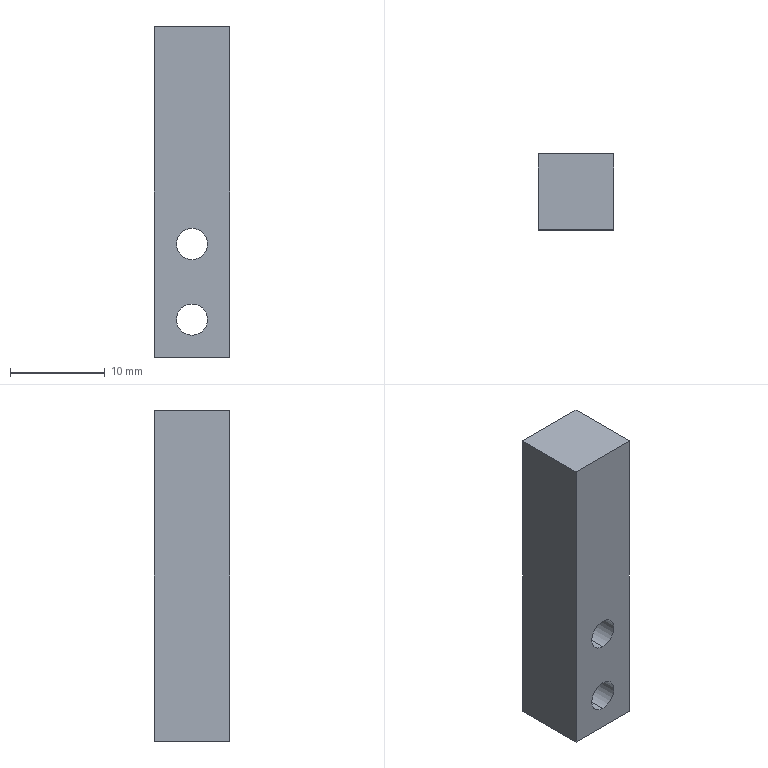Part | SolidWorks | features Extrusion 1, HoleWzd 1 | 1 solid | 10 faces | box 8 x 8 x 35 mm | volume 2103 mm3 | plane 6 | cylinder 4 | commonest cylinder face diameters 3.3 x4
STEP:
#1=CARTESIAN_POINT('',(0.,4.,13.65));
#2=VERTEX_POINT('',#1);
#3=CARTESIAN_POINT('',(0.,4.,10.35));
#4=VERTEX_POINT('',#3);
#5=CARTESIAN_POINT('',(0.,4.,12.));
#6=DIRECTION('',(0.,-1.,0.));
#7=DIRECTION('',(0.,0.,-1.));
#8=AXIS2_PLACEMENT_3D('',#5,#6,#7);
#9=CIRCLE('',#8,1.65);
#10=EDGE_CURVE('',#2,#4,#9,.T.);
#11=ORIENTED_EDGE('',*,*,#10,.F.);
#12=CARTESIAN_POINT('',(0.,-4.,13.65));
#13=VERTEX_POINT('',#12);
#14=CARTESIAN_POINT('',(0.,-4.,13.65));
#15=DIRECTION('',(0.,-1.,0.));
#16=VECTOR('',#15,1000.);
#17=LINE('',#14,#16);
#18=EDGE_CURVE('',#2,#13,#17,.T.);
#19=ORIENTED_EDGE('',*,*,#18,.T.);
#20=CARTESIAN_POINT('',(0.,-4.,10.35));
#21=VERTEX_POINT('',#20);
#22=CARTESIAN_POINT('',(0.,-4.,12.));
#23=DIRECTION('',(0.,-1.,0.));
#24=DIRECTION('',(0.,0.,-1.));
#25=AXIS2_PLACEMENT_3D('',#22,#23,#24);
#26=CIRCLE('',#25,1.65);
#27=EDGE_CURVE('',#13,#21,#26,.T.);
#28=ORIENTED_EDGE('',*,*,#27,.T.);
#29=CARTESIAN_POINT('',(0.,-4.,10.35));
#30=DIRECTION('',(0.,-1.,0.));
#31=VECTOR('',#30,1000.);
#32=LINE('',#29,#31);
#33=EDGE_CURVE('',#4,#21,#32,.T.);
#34=ORIENTED_EDGE('',*,*,#33,.F.);
#35=EDGE_LOOP('',(#11,#19,#28,#34));
#36=FACE_OUTER_BOUND('',#35,.T.);
#37=CARTESIAN_POINT('',(0.,-4.,12.));
#38=DIRECTION('',(0.,-1.,0.));
#39=DIRECTION('',(0.,0.,-1.));
#40=AXIS2_PLACEMENT_3D('',#37,#38,#39);
#41=CYLINDRICAL_SURFACE('',#40,1.65);
#42=ADVANCED_FACE('',(#36),#41,.F.);
#43=CARTESIAN_POINT('',(0.,4.,5.65));
#44=VERTEX_POINT('',#43);
#45=CARTESIAN_POINT('',(0.,4.,2.35));
#46=VERTEX_POINT('',#45);
#47=CARTESIAN_POINT('',(0.,4.,4.));
#48=DIRECTION('',(0.,-1.,0.));
#49=DIRECTION('',(0.,0.,-1.));
#50=AXIS2_PLACEMENT_3D('',#47,#48,#49);
#51=CIRCLE('',#50,1.65);
#52=EDGE_CURVE('',#44,#46,#51,.T.);
#53=ORIENTED_EDGE('',*,*,#52,.F.);
#54=CARTESIAN_POINT('',(0.,-4.,5.65));
#55=VERTEX_POINT('',#54);
#56=CARTESIAN_POINT('',(0.,-4.,5.65));
#57=DIRECTION('',(0.,-1.,0.));
#58=VECTOR('',#57,1000.);
#59=LINE('',#56,#58);
#60=EDGE_CURVE('',#44,#55,#59,.T.);
#61=ORIENTED_EDGE('',*,*,#60,.T.);
#62=CARTESIAN_POINT('',(0.,-4.,2.35));
#63=VERTEX_POINT('',#62);
#64=CARTESIAN_POINT('',(0.,-4.,4.));
#65=DIRECTION('',(0.,-1.,0.));
#66=DIRECTION('',(0.,0.,-1.));
#67=AXIS2_PLACEMENT_3D('',#64,#65,#66);
#68=CIRCLE('',#67,1.65);
#69=EDGE_CURVE('',#55,#63,#68,.T.);
#70=ORIENTED_EDGE('',*,*,#69,.T.);
#71=CARTESIAN_POINT('',(0.,-4.,2.35));
#72=DIRECTION('',(0.,-1.,0.));
#73=VECTOR('',#72,1000.);
#74=LINE('',#71,#73);
#75=EDGE_CURVE('',#46,#63,#74,.T.);
#76=ORIENTED_EDGE('',*,*,#75,.F.);
#77=EDGE_LOOP('',(#53,#61,#70,#76));
#78=FACE_OUTER_BOUND('',#77,.T.);
#79=CARTESIAN_POINT('',(0.,-4.,4.));
#80=DIRECTION('',(0.,-1.,0.));
#81=DIRECTION('',(0.,0.,-1.));
#82=AXIS2_PLACEMENT_3D('',#79,#80,#81);
#83=CYLINDRICAL_SURFACE('',#82,1.65);
#84=ADVANCED_FACE('',(#78),#83,.F.);
#85=CARTESIAN_POINT('',(4.,-4.,0.));
#86=VERTEX_POINT('',#85);
#87=CARTESIAN_POINT('',(4.,4.,0.));
#88=VERTEX_POINT('',#87);
#89=CARTESIAN_POINT('',(4.,4.,0.));
#90=DIRECTION('',(0.,1.,0.));
#91=VECTOR('',#90,1000.);
#92=LINE('',#89,#91);
#93=EDGE_CURVE('',#86,#88,#92,.T.);
#94=ORIENTED_EDGE('',*,*,#93,.T.);
#95=CARTESIAN_POINT('',(4.,4.,35.));
#96=VERTEX_POINT('',#95);
#97=CARTESIAN_POINT('',(4.,4.,35.));
#98=DIRECTION('',(0.,0.,-1.));
#99=VECTOR('',#98,1000.);
#100=LINE('',#97,#99);
#101=EDGE_CURVE('',#96,#88,#100,.T.);
#102=ORIENTED_EDGE('',*,*,#101,.F.);
#103=CARTESIAN_POINT('',(4.,-4.,35.));
#104=VERTEX_POINT('',#103);
#105=CARTESIAN_POINT('',(4.,4.,35.));
#106=DIRECTION('',(0.,1.,0.));
#107=VECTOR('',#106,1000.);
#108=LINE('',#105,#107);
#109=EDGE_CURVE('',#104,#96,#108,.T.);
#110=ORIENTED_EDGE('',*,*,#109,.F.);
#111=CARTESIAN_POINT('',(4.,-4.,35.));
#112=DIRECTION('',(0.,0.,-1.));
#113=VECTOR('',#112,1000.);
#114=LINE('',#111,#113);
#115=EDGE_CURVE('',#104,#86,#114,.T.);
#116=ORIENTED_EDGE('',*,*,#115,.T.);
#117=EDGE_LOOP('',(#94,#102,#110,#116));
#118=FACE_OUTER_BOUND('',#117,.T.);
#119=CARTESIAN_POINT('',(4.,4.,35.));
#120=DIRECTION('',(-1.,0.,0.));
#121=DIRECTION('',(0.,-1.,0.));
#122=AXIS2_PLACEMENT_3D('',#119,#120,#121);
#123=PLANE('',#122);
#124=ADVANCED_FACE('',(#118),#123,.F.);
#125=CARTESIAN_POINT('',(0.,4.,12.));
#126=DIRECTION('',(0.,-1.,0.));
#127=DIRECTION('',(0.,0.,-1.));
#128=AXIS2_PLACEMENT_3D('',#125,#126,#127);
#129=CIRCLE('',#128,1.65);
#130=EDGE_CURVE('',#4,#2,#129,.T.);
#131=ORIENTED_EDGE('',*,*,#130,.T.);
#132=ORIENTED_EDGE('',*,*,#10,.T.);
#133=EDGE_LOOP('',(#131,#132));
#134=FACE_BOUND('',#133,.T.);
#135=CARTESIAN_POINT('',(0.,4.,4.));
#136=DIRECTION('',(0.,-1.,0.));
#137=DIRECTION('',(0.,0.,-1.));
#138=AXIS2_PLACEMENT_3D('',#135,#136,#137);
#139=CIRCLE('',#138,1.65);
#140=EDGE_CURVE('',#46,#44,#139,.T.);
#141=ORIENTED_EDGE('',*,*,#140,.T.);
#142=ORIENTED_EDGE('',*,*,#52,.T.);
#143=EDGE_LOOP('',(#141,#142));
#144=FACE_BOUND('',#143,.T.);
#145=CARTESIAN_POINT('',(-4.,4.,0.));
#146=VERTEX_POINT('',#145);
#147=CARTESIAN_POINT('',(-4.,4.,0.));
#148=DIRECTION('',(-1.,0.,0.));
#149=VECTOR('',#148,1000.);
#150=LINE('',#147,#149);
#151=EDGE_CURVE('',#88,#146,#150,.T.);
#152=ORIENTED_EDGE('',*,*,#151,.T.);
#153=CARTESIAN_POINT('',(-4.,4.,35.));
#154=VERTEX_POINT('',#153);
#155=CARTESIAN_POINT('',(-4.,4.,35.));
#156=DIRECTION('',(0.,0.,-1.));
#157=VECTOR('',#156,1000.);
#158=LINE('',#155,#157);
#159=EDGE_CURVE('',#154,#146,#158,.T.);
#160=ORIENTED_EDGE('',*,*,#159,.F.);
#161=CARTESIAN_POINT('',(-4.,4.,35.));
#162=DIRECTION('',(-1.,0.,0.));
#163=VECTOR('',#162,1000.);
#164=LINE('',#161,#163);
#165=EDGE_CURVE('',#96,#154,#164,.T.);
#166=ORIENTED_EDGE('',*,*,#165,.F.);
#167=ORIENTED_EDGE('',*,*,#101,.T.);
#168=EDGE_LOOP('',(#152,#160,#166,#167));
#169=FACE_OUTER_BOUND('',#168,.T.);
#170=CARTESIAN_POINT('',(-4.,4.,35.));
#171=DIRECTION('',(0.,-1.,0.));
#172=DIRECTION('',(0.,0.,-1.));
#173=AXIS2_PLACEMENT_3D('',#170,#171,#172);
#174=PLANE('',#173);
#175=ADVANCED_FACE('',(#134,#144,#169),#174,.F.);
#176=CARTESIAN_POINT('',(-4.,-4.,0.));
#177=VERTEX_POINT('',#176);
#178=CARTESIAN_POINT('',(-4.,4.,0.));
#179=DIRECTION('',(0.,-1.,0.));
#180=VECTOR('',#179,1000.);
#181=LINE('',#178,#180);
#182=EDGE_CURVE('',#146,#177,#181,.T.);
#183=ORIENTED_EDGE('',*,*,#182,.T.);
#184=CARTESIAN_POINT('',(-4.,-4.,35.));
#185=VERTEX_POINT('',#184);
#186=CARTESIAN_POINT('',(-4.,-4.,35.));
#187=DIRECTION('',(0.,0.,-1.));
#188=VECTOR('',#187,1000.);
#189=LINE('',#186,#188);
#190=EDGE_CURVE('',#185,#177,#189,.T.);
#191=ORIENTED_EDGE('',*,*,#190,.F.);
#192=CARTESIAN_POINT('',(-4.,4.,35.));
#193=DIRECTION('',(0.,-1.,0.));
#194=VECTOR('',#193,1000.);
#195=LINE('',#192,#194);
#196=EDGE_CURVE('',#154,#185,#195,.T.);
#197=ORIENTED_EDGE('',*,*,#196,.F.);
#198=ORIENTED_EDGE('',*,*,#159,.T.);
#199=EDGE_LOOP('',(#183,#191,#197,#198));
#200=FACE_OUTER_BOUND('',#199,.T.);
#201=CARTESIAN_POINT('',(-4.,4.,35.));
#202=DIRECTION('',(1.,0.,0.));
#203=DIRECTION('',(0.,1.,0.));
#204=AXIS2_PLACEMENT_3D('',#201,#202,#203);
#205=PLANE('',#204);
#206=ADVANCED_FACE('',(#200),#205,.F.);
#207=CARTESIAN_POINT('',(0.,-4.,12.));
#208=DIRECTION('',(0.,-1.,0.));
#209=DIRECTION('',(0.,0.,-1.));
#210=AXIS2_PLACEMENT_3D('',#207,#208,#209);
#211=CIRCLE('',#210,1.65);
#212=EDGE_CURVE('',#21,#13,#211,.T.);
#213=ORIENTED_EDGE('',*,*,#212,.F.);
#214=ORIENTED_EDGE('',*,*,#27,.F.);
#215=EDGE_LOOP('',(#213,#214));
#216=FACE_BOUND('',#215,.T.);
#217=CARTESIAN_POINT('',(0.,-4.,4.));
#218=DIRECTION('',(0.,-1.,0.));
#219=DIRECTION('',(0.,0.,-1.));
#220=AXIS2_PLACEMENT_3D('',#217,#218,#219);
#221=CIRCLE('',#220,1.65);
#222=EDGE_CURVE('',#63,#55,#221,.T.);
#223=ORIENTED_EDGE('',*,*,#222,.F.);
#224=ORIENTED_EDGE('',*,*,#69,.F.);
#225=EDGE_LOOP('',(#223,#224));
#226=FACE_BOUND('',#225,.T.);
#227=CARTESIAN_POINT('',(-4.,-4.,0.));
#228=DIRECTION('',(1.,0.,0.));
#229=VECTOR('',#228,1000.);
#230=LINE('',#227,#229);
#231=EDGE_CURVE('',#177,#86,#230,.T.);
#232=ORIENTED_EDGE('',*,*,#231,.T.);
#233=ORIENTED_EDGE('',*,*,#115,.F.);
#234=CARTESIAN_POINT('',(-4.,-4.,35.));
#235=DIRECTION('',(1.,0.,0.));
#236=VECTOR('',#235,1000.);
#237=LINE('',#234,#236);
#238=EDGE_CURVE('',#185,#104,#237,.T.);
#239=ORIENTED_EDGE('',*,*,#238,.F.);
#240=ORIENTED_EDGE('',*,*,#190,.T.);
#241=EDGE_LOOP('',(#232,#233,#239,#240));
#242=FACE_OUTER_BOUND('',#241,.T.);
#243=CARTESIAN_POINT('',(-4.,-4.,35.));
#244=DIRECTION('',(0.,1.,0.));
#245=DIRECTION('',(0.,0.,1.));
#246=AXIS2_PLACEMENT_3D('',#243,#244,#245);
#247=PLANE('',#246);
#248=ADVANCED_FACE('',(#216,#226,#242),#247,.F.);
#249=ORIENTED_EDGE('',*,*,#109,.T.);
#250=ORIENTED_EDGE('',*,*,#165,.T.);
#251=ORIENTED_EDGE('',*,*,#196,.T.);
#252=ORIENTED_EDGE('',*,*,#238,.T.);
#253=EDGE_LOOP('',(#249,#250,#251,#252));
#254=FACE_OUTER_BOUND('',#253,.T.);
#255=CARTESIAN_POINT('',(0.,0.,35.));
#256=DIRECTION('',(0.,0.,1.));
#257=DIRECTION('',(1.,0.,0.));
#258=AXIS2_PLACEMENT_3D('',#255,#256,#257);
#259=PLANE('',#258);
#260=ADVANCED_FACE('',(#254),#259,.T.);
#261=ORIENTED_EDGE('',*,*,#93,.F.);
#262=ORIENTED_EDGE('',*,*,#231,.F.);
#263=ORIENTED_EDGE('',*,*,#182,.F.);
#264=ORIENTED_EDGE('',*,*,#151,.F.);
#265=EDGE_LOOP('',(#261,#262,#263,#264));
#266=FACE_OUTER_BOUND('',#265,.T.);
#267=CARTESIAN_POINT('',(0.,0.,0.));
#268=DIRECTION('',(0.,0.,1.));
#269=DIRECTION('',(1.,0.,0.));
#270=AXIS2_PLACEMENT_3D('',#267,#268,#269);
#271=PLANE('',#270);
#272=ADVANCED_FACE('',(#266),#271,.F.);
#273=ORIENTED_EDGE('',*,*,#60,.F.);
#274=ORIENTED_EDGE('',*,*,#140,.F.);
#275=ORIENTED_EDGE('',*,*,#75,.T.);
#276=ORIENTED_EDGE('',*,*,#222,.T.);
#277=EDGE_LOOP('',(#273,#274,#275,#276));
#278=FACE_OUTER_BOUND('',#277,.T.);
#279=CARTESIAN_POINT('',(0.,-4.,4.));
#280=DIRECTION('',(0.,-1.,0.));
#281=DIRECTION('',(0.,0.,-1.));
#282=AXIS2_PLACEMENT_3D('',#279,#280,#281);
#283=CYLINDRICAL_SURFACE('',#282,1.65);
#284=ADVANCED_FACE('',(#278),#283,.F.);
#285=ORIENTED_EDGE('',*,*,#18,.F.);
#286=ORIENTED_EDGE('',*,*,#130,.F.);
#287=ORIENTED_EDGE('',*,*,#33,.T.);
#288=ORIENTED_EDGE('',*,*,#212,.T.);
#289=EDGE_LOOP('',(#285,#286,#287,#288));
#290=FACE_OUTER_BOUND('',#289,.T.);
#291=CARTESIAN_POINT('',(0.,-4.,12.));
#292=DIRECTION('',(0.,-1.,0.));
#293=DIRECTION('',(0.,0.,-1.));
#294=AXIS2_PLACEMENT_3D('',#291,#292,#293);
#295=CYLINDRICAL_SURFACE('',#294,1.65);
#296=ADVANCED_FACE('',(#290),#295,.F.);
#297=CLOSED_SHELL('',(#42,#84,#124,#175,#206,#248,#260,#272,#284,#296));
#298=MANIFOLD_SOLID_BREP('',#297);
#299=CARTESIAN_POINT('',(0.,0.,0.));
#300=DIRECTION('',(0.,0.,1.));
#301=DIRECTION('',(1.,0.,0.));
#302=AXIS2_PLACEMENT_3D('',#299,#300,#301);
#303=(LENGTH_UNIT()NAMED_UNIT(*)SI_UNIT(.MILLI.,.METRE.));
#304=UNCERTAINTY_MEASURE_WITH_UNIT(LENGTH_MEASURE(0.00001),#303,'','');
#305=(NAMED_UNIT(*)PLANE_ANGLE_UNIT()SI_UNIT($,.RADIAN.));
#306=(NAMED_UNIT(*)SI_UNIT($,.STERADIAN.)SOLID_ANGLE_UNIT());
#307=(GEOMETRIC_REPRESENTATION_CONTEXT(3)GLOBAL_UNCERTAINTY_ASSIGNED_CONTEXT((#304))GLOBAL_UNIT_ASSIGNED_CONTEXT((#303,#305,#306))REPRESENTATION_CONTEXT('',''));
#308=ADVANCED_BREP_SHAPE_REPRESENTATION('',(#298,#302),#307);